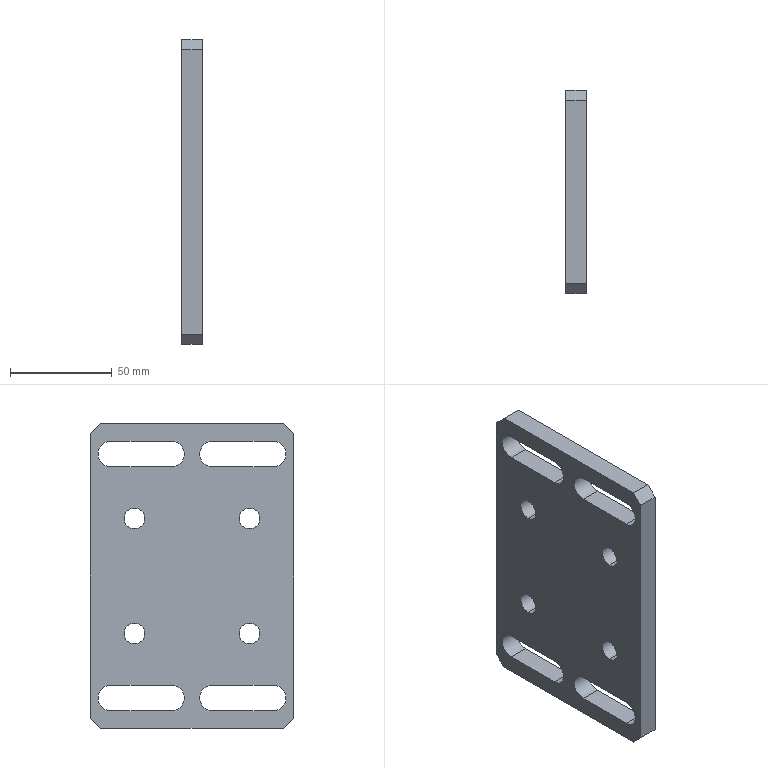Part | SolidWorks | features Chamfer 1, Extrusion 1, HoleWzd 1, ICE 1 | 1 solid | 34 faces | box 10 x 100 x 150 mm | volume 126323 mm3 | plane 18 | cylinder 16 | commonest cylinder face diameters 10.2 x8 12.5 x8
STEP:
#1=CARTESIAN_POINT('',(0.,28.284,33.384));
#2=VERTEX_POINT('',#1);
#3=CARTESIAN_POINT('',(0.,28.284,23.184));
#4=VERTEX_POINT('',#3);
#5=CARTESIAN_POINT('',(0.,28.284,28.284));
#6=DIRECTION('',(1.,0.,0.));
#7=DIRECTION('',(0.,0.,-1.));
#8=AXIS2_PLACEMENT_3D('',#5,#6,#7);
#9=CIRCLE('',#8,5.1);
#10=EDGE_CURVE('',#2,#4,#9,.T.);
#11=ORIENTED_EDGE('',*,*,#10,.F.);
#12=CARTESIAN_POINT('',(10.,28.284,33.384));
#13=VERTEX_POINT('',#12);
#14=CARTESIAN_POINT('',(10.,28.284,33.384));
#15=DIRECTION('',(1.,0.,0.));
#16=VECTOR('',#15,1000.);
#17=LINE('',#14,#16);
#18=EDGE_CURVE('',#2,#13,#17,.T.);
#19=ORIENTED_EDGE('',*,*,#18,.T.);
#20=CARTESIAN_POINT('',(10.,28.284,23.184));
#21=VERTEX_POINT('',#20);
#22=CARTESIAN_POINT('',(10.,28.284,28.284));
#23=DIRECTION('',(1.,0.,0.));
#24=DIRECTION('',(0.,0.,-1.));
#25=AXIS2_PLACEMENT_3D('',#22,#23,#24);
#26=CIRCLE('',#25,5.1);
#27=EDGE_CURVE('',#13,#21,#26,.T.);
#28=ORIENTED_EDGE('',*,*,#27,.T.);
#29=CARTESIAN_POINT('',(10.,28.284,23.184));
#30=DIRECTION('',(1.,0.,0.));
#31=VECTOR('',#30,1000.);
#32=LINE('',#29,#31);
#33=EDGE_CURVE('',#4,#21,#32,.T.);
#34=ORIENTED_EDGE('',*,*,#33,.F.);
#35=EDGE_LOOP('',(#11,#19,#28,#34));
#36=FACE_OUTER_BOUND('',#35,.T.);
#37=CARTESIAN_POINT('',(10.,28.284,28.284));
#38=DIRECTION('',(1.,0.,0.));
#39=DIRECTION('',(0.,0.,-1.));
#40=AXIS2_PLACEMENT_3D('',#37,#38,#39);
#41=CYLINDRICAL_SURFACE('',#40,5.1);
#42=ADVANCED_FACE('',(#36),#41,.F.);
#43=CARTESIAN_POINT('',(0.,28.284,-23.184));
#44=VERTEX_POINT('',#43);
#45=CARTESIAN_POINT('',(0.,28.284,-33.384));
#46=VERTEX_POINT('',#45);
#47=CARTESIAN_POINT('',(0.,28.284,-28.284));
#48=DIRECTION('',(1.,0.,0.));
#49=DIRECTION('',(0.,0.,-1.));
#50=AXIS2_PLACEMENT_3D('',#47,#48,#49);
#51=CIRCLE('',#50,5.1);
#52=EDGE_CURVE('',#44,#46,#51,.T.);
#53=ORIENTED_EDGE('',*,*,#52,.F.);
#54=CARTESIAN_POINT('',(10.,28.284,-23.184));
#55=VERTEX_POINT('',#54);
#56=CARTESIAN_POINT('',(10.,28.284,-23.184));
#57=DIRECTION('',(1.,0.,0.));
#58=VECTOR('',#57,1000.);
#59=LINE('',#56,#58);
#60=EDGE_CURVE('',#44,#55,#59,.T.);
#61=ORIENTED_EDGE('',*,*,#60,.T.);
#62=CARTESIAN_POINT('',(10.,28.284,-33.384));
#63=VERTEX_POINT('',#62);
#64=CARTESIAN_POINT('',(10.,28.284,-28.284));
#65=DIRECTION('',(1.,0.,0.));
#66=DIRECTION('',(0.,0.,-1.));
#67=AXIS2_PLACEMENT_3D('',#64,#65,#66);
#68=CIRCLE('',#67,5.1);
#69=EDGE_CURVE('',#55,#63,#68,.T.);
#70=ORIENTED_EDGE('',*,*,#69,.T.);
#71=CARTESIAN_POINT('',(10.,28.284,-33.384));
#72=DIRECTION('',(1.,0.,0.));
#73=VECTOR('',#72,1000.);
#74=LINE('',#71,#73);
#75=EDGE_CURVE('',#46,#63,#74,.T.);
#76=ORIENTED_EDGE('',*,*,#75,.F.);
#77=EDGE_LOOP('',(#53,#61,#70,#76));
#78=FACE_OUTER_BOUND('',#77,.T.);
#79=CARTESIAN_POINT('',(10.,28.284,-28.284));
#80=DIRECTION('',(1.,0.,0.));
#81=DIRECTION('',(0.,0.,-1.));
#82=AXIS2_PLACEMENT_3D('',#79,#80,#81);
#83=CYLINDRICAL_SURFACE('',#82,5.1);
#84=ADVANCED_FACE('',(#78),#83,.F.);
#85=CARTESIAN_POINT('',(0.,-28.284,-23.184));
#86=VERTEX_POINT('',#85);
#87=CARTESIAN_POINT('',(0.,-28.284,-33.384));
#88=VERTEX_POINT('',#87);
#89=CARTESIAN_POINT('',(0.,-28.284,-28.284));
#90=DIRECTION('',(1.,0.,0.));
#91=DIRECTION('',(0.,0.,-1.));
#92=AXIS2_PLACEMENT_3D('',#89,#90,#91);
#93=CIRCLE('',#92,5.1);
#94=EDGE_CURVE('',#86,#88,#93,.T.);
#95=ORIENTED_EDGE('',*,*,#94,.F.);
#96=CARTESIAN_POINT('',(10.,-28.284,-23.184));
#97=VERTEX_POINT('',#96);
#98=CARTESIAN_POINT('',(10.,-28.284,-23.184));
#99=DIRECTION('',(1.,0.,0.));
#100=VECTOR('',#99,1000.);
#101=LINE('',#98,#100);
#102=EDGE_CURVE('',#86,#97,#101,.T.);
#103=ORIENTED_EDGE('',*,*,#102,.T.);
#104=CARTESIAN_POINT('',(10.,-28.284,-33.384));
#105=VERTEX_POINT('',#104);
#106=CARTESIAN_POINT('',(10.,-28.284,-28.284));
#107=DIRECTION('',(1.,0.,0.));
#108=DIRECTION('',(0.,0.,-1.));
#109=AXIS2_PLACEMENT_3D('',#106,#107,#108);
#110=CIRCLE('',#109,5.1);
#111=EDGE_CURVE('',#97,#105,#110,.T.);
#112=ORIENTED_EDGE('',*,*,#111,.T.);
#113=CARTESIAN_POINT('',(10.,-28.284,-33.384));
#114=DIRECTION('',(1.,0.,0.));
#115=VECTOR('',#114,1000.);
#116=LINE('',#113,#115);
#117=EDGE_CURVE('',#88,#105,#116,.T.);
#118=ORIENTED_EDGE('',*,*,#117,.F.);
#119=EDGE_LOOP('',(#95,#103,#112,#118));
#120=FACE_OUTER_BOUND('',#119,.T.);
#121=CARTESIAN_POINT('',(10.,-28.284,-28.284));
#122=DIRECTION('',(1.,0.,0.));
#123=DIRECTION('',(0.,0.,-1.));
#124=AXIS2_PLACEMENT_3D('',#121,#122,#123);
#125=CYLINDRICAL_SURFACE('',#124,5.1);
#126=ADVANCED_FACE('',(#120),#125,.F.);
#127=CARTESIAN_POINT('',(0.,-28.284,33.384));
#128=VERTEX_POINT('',#127);
#129=CARTESIAN_POINT('',(0.,-28.284,23.184));
#130=VERTEX_POINT('',#129);
#131=CARTESIAN_POINT('',(0.,-28.284,28.284));
#132=DIRECTION('',(1.,0.,0.));
#133=DIRECTION('',(0.,0.,-1.));
#134=AXIS2_PLACEMENT_3D('',#131,#132,#133);
#135=CIRCLE('',#134,5.1);
#136=EDGE_CURVE('',#128,#130,#135,.T.);
#137=ORIENTED_EDGE('',*,*,#136,.F.);
#138=CARTESIAN_POINT('',(10.,-28.284,33.384));
#139=VERTEX_POINT('',#138);
#140=CARTESIAN_POINT('',(10.,-28.284,33.384));
#141=DIRECTION('',(1.,0.,0.));
#142=VECTOR('',#141,1000.);
#143=LINE('',#140,#142);
#144=EDGE_CURVE('',#128,#139,#143,.T.);
#145=ORIENTED_EDGE('',*,*,#144,.T.);
#146=CARTESIAN_POINT('',(10.,-28.284,23.184));
#147=VERTEX_POINT('',#146);
#148=CARTESIAN_POINT('',(10.,-28.284,28.284));
#149=DIRECTION('',(1.,0.,0.));
#150=DIRECTION('',(0.,0.,-1.));
#151=AXIS2_PLACEMENT_3D('',#148,#149,#150);
#152=CIRCLE('',#151,5.1);
#153=EDGE_CURVE('',#139,#147,#152,.T.);
#154=ORIENTED_EDGE('',*,*,#153,.T.);
#155=CARTESIAN_POINT('',(10.,-28.284,23.184));
#156=DIRECTION('',(1.,0.,0.));
#157=VECTOR('',#156,1000.);
#158=LINE('',#155,#157);
#159=EDGE_CURVE('',#130,#147,#158,.T.);
#160=ORIENTED_EDGE('',*,*,#159,.F.);
#161=EDGE_LOOP('',(#137,#145,#154,#160));
#162=FACE_OUTER_BOUND('',#161,.T.);
#163=CARTESIAN_POINT('',(10.,-28.284,28.284));
#164=DIRECTION('',(1.,0.,0.));
#165=DIRECTION('',(0.,0.,-1.));
#166=AXIS2_PLACEMENT_3D('',#163,#164,#165);
#167=CYLINDRICAL_SURFACE('',#166,5.1);
#168=ADVANCED_FACE('',(#162),#167,.F.);
#169=CARTESIAN_POINT('',(0.,-45.,-75.));
#170=VERTEX_POINT('',#169);
#171=CARTESIAN_POINT('',(0.,45.,-75.));
#172=VERTEX_POINT('',#171);
#173=CARTESIAN_POINT('',(0.,50.,-75.));
#174=DIRECTION('',(0.,1.,0.));
#175=VECTOR('',#174,1000.);
#176=LINE('',#173,#175);
#177=EDGE_CURVE('',#170,#172,#176,.T.);
#178=ORIENTED_EDGE('',*,*,#177,.T.);
#179=CARTESIAN_POINT('',(10.,45.,-75.));
#180=VERTEX_POINT('',#179);
#181=CARTESIAN_POINT('',(10.,45.,-75.));
#182=DIRECTION('',(1.,0.,0.));
#183=VECTOR('',#182,1000.);
#184=LINE('',#181,#183);
#185=EDGE_CURVE('',#172,#180,#184,.T.);
#186=ORIENTED_EDGE('',*,*,#185,.T.);
#187=CARTESIAN_POINT('',(10.,-45.,-75.));
#188=VERTEX_POINT('',#187);
#189=CARTESIAN_POINT('',(10.,50.,-75.));
#190=DIRECTION('',(0.,1.,0.));
#191=VECTOR('',#190,1000.);
#192=LINE('',#189,#191);
#193=EDGE_CURVE('',#188,#180,#192,.T.);
#194=ORIENTED_EDGE('',*,*,#193,.F.);
#195=CARTESIAN_POINT('',(10.,-45.,-75.));
#196=DIRECTION('',(-1.,0.,0.));
#197=VECTOR('',#196,1000.);
#198=LINE('',#195,#197);
#199=EDGE_CURVE('',#188,#170,#198,.T.);
#200=ORIENTED_EDGE('',*,*,#199,.T.);
#201=EDGE_LOOP('',(#178,#186,#194,#200));
#202=FACE_OUTER_BOUND('',#201,.T.);
#203=CARTESIAN_POINT('',(10.,50.,-75.));
#204=DIRECTION('',(0.,0.,1.));
#205=DIRECTION('',(0.,-1.,0.));
#206=AXIS2_PLACEMENT_3D('',#203,#204,#205);
#207=PLANE('',#206);
#208=ADVANCED_FACE('',(#202),#207,.F.);
#209=CARTESIAN_POINT('',(0.,50.,-70.));
#210=VERTEX_POINT('',#209);
#211=CARTESIAN_POINT('',(0.,50.,70.));
#212=VERTEX_POINT('',#211);
#213=CARTESIAN_POINT('',(0.,50.,75.));
#214=DIRECTION('',(0.,0.,1.));
#215=VECTOR('',#214,1000.);
#216=LINE('',#213,#215);
#217=EDGE_CURVE('',#210,#212,#216,.T.);
#218=ORIENTED_EDGE('',*,*,#217,.T.);
#219=CARTESIAN_POINT('',(10.,50.,70.));
#220=VERTEX_POINT('',#219);
#221=CARTESIAN_POINT('',(10.,50.,70.));
#222=DIRECTION('',(1.,0.,0.));
#223=VECTOR('',#222,1000.);
#224=LINE('',#221,#223);
#225=EDGE_CURVE('',#212,#220,#224,.T.);
#226=ORIENTED_EDGE('',*,*,#225,.T.);
#227=CARTESIAN_POINT('',(10.,50.,-70.));
#228=VERTEX_POINT('',#227);
#229=CARTESIAN_POINT('',(10.,50.,75.));
#230=DIRECTION('',(0.,0.,1.));
#231=VECTOR('',#230,1000.);
#232=LINE('',#229,#231);
#233=EDGE_CURVE('',#228,#220,#232,.T.);
#234=ORIENTED_EDGE('',*,*,#233,.F.);
#235=CARTESIAN_POINT('',(10.,50.,-70.));
#236=DIRECTION('',(-1.,0.,0.));
#237=VECTOR('',#236,1000.);
#238=LINE('',#235,#237);
#239=EDGE_CURVE('',#228,#210,#238,.T.);
#240=ORIENTED_EDGE('',*,*,#239,.T.);
#241=EDGE_LOOP('',(#218,#226,#234,#240));
#242=FACE_OUTER_BOUND('',#241,.T.);
#243=CARTESIAN_POINT('',(10.,50.,75.));
#244=DIRECTION('',(0.,-1.,0.));
#245=DIRECTION('',(0.,0.,-1.));
#246=AXIS2_PLACEMENT_3D('',#243,#244,#245);
#247=PLANE('',#246);
#248=ADVANCED_FACE('',(#242),#247,.F.);
#249=CARTESIAN_POINT('',(0.,45.,75.));
#250=VERTEX_POINT('',#249);
#251=CARTESIAN_POINT('',(0.,-45.,75.));
#252=VERTEX_POINT('',#251);
#253=CARTESIAN_POINT('',(0.,50.,75.));
#254=DIRECTION('',(0.,-1.,0.));
#255=VECTOR('',#254,1000.);
#256=LINE('',#253,#255);
#257=EDGE_CURVE('',#250,#252,#256,.T.);
#258=ORIENTED_EDGE('',*,*,#257,.T.);
#259=CARTESIAN_POINT('',(10.,-45.,75.));
#260=VERTEX_POINT('',#259);
#261=CARTESIAN_POINT('',(10.,-45.,75.));
#262=DIRECTION('',(1.,0.,0.));
#263=VECTOR('',#262,1000.);
#264=LINE('',#261,#263);
#265=EDGE_CURVE('',#252,#260,#264,.T.);
#266=ORIENTED_EDGE('',*,*,#265,.T.);
#267=CARTESIAN_POINT('',(10.,45.,75.));
#268=VERTEX_POINT('',#267);
#269=CARTESIAN_POINT('',(10.,50.,75.));
#270=DIRECTION('',(0.,-1.,0.));
#271=VECTOR('',#270,1000.);
#272=LINE('',#269,#271);
#273=EDGE_CURVE('',#268,#260,#272,.T.);
#274=ORIENTED_EDGE('',*,*,#273,.F.);
#275=CARTESIAN_POINT('',(10.,45.,75.));
#276=DIRECTION('',(-1.,0.,0.));
#277=VECTOR('',#276,1000.);
#278=LINE('',#275,#277);
#279=EDGE_CURVE('',#268,#250,#278,.T.);
#280=ORIENTED_EDGE('',*,*,#279,.T.);
#281=EDGE_LOOP('',(#258,#266,#274,#280));
#282=FACE_OUTER_BOUND('',#281,.T.);
#283=CARTESIAN_POINT('',(10.,50.,75.));
#284=DIRECTION('',(0.,0.,-1.));
#285=DIRECTION('',(0.,1.,0.));
#286=AXIS2_PLACEMENT_3D('',#283,#284,#285);
#287=PLANE('',#286);
#288=ADVANCED_FACE('',(#282),#287,.F.);
#289=CARTESIAN_POINT('',(10.,-50.,70.));
#290=VERTEX_POINT('',#289);
#291=CARTESIAN_POINT('',(10.,-50.,-70.));
#292=VERTEX_POINT('',#291);
#293=CARTESIAN_POINT('',(10.,-50.,75.));
#294=DIRECTION('',(0.,0.,-1.));
#295=VECTOR('',#294,1000.);
#296=LINE('',#293,#295);
#297=EDGE_CURVE('',#290,#292,#296,.T.);
#298=ORIENTED_EDGE('',*,*,#297,.F.);
#299=CARTESIAN_POINT('',(0.,-50.,70.));
#300=VERTEX_POINT('',#299);
#301=CARTESIAN_POINT('',(10.,-50.,70.));
#302=DIRECTION('',(-1.,0.,0.));
#303=VECTOR('',#302,1000.);
#304=LINE('',#301,#303);
#305=EDGE_CURVE('',#290,#300,#304,.T.);
#306=ORIENTED_EDGE('',*,*,#305,.T.);
#307=CARTESIAN_POINT('',(0.,-50.,-70.));
#308=VERTEX_POINT('',#307);
#309=CARTESIAN_POINT('',(0.,-50.,75.));
#310=DIRECTION('',(0.,0.,-1.));
#311=VECTOR('',#310,1000.);
#312=LINE('',#309,#311);
#313=EDGE_CURVE('',#300,#308,#312,.T.);
#314=ORIENTED_EDGE('',*,*,#313,.T.);
#315=CARTESIAN_POINT('',(10.,-50.,-70.));
#316=DIRECTION('',(1.,0.,0.));
#317=VECTOR('',#316,1000.);
#318=LINE('',#315,#317);
#319=EDGE_CURVE('',#308,#292,#318,.T.);
#320=ORIENTED_EDGE('',*,*,#319,.T.);
#321=EDGE_LOOP('',(#298,#306,#314,#320));
#322=FACE_OUTER_BOUND('',#321,.T.);
#323=CARTESIAN_POINT('',(10.,-50.,75.));
#324=DIRECTION('',(0.,1.,0.));
#325=DIRECTION('',(0.,0.,1.));
#326=AXIS2_PLACEMENT_3D('',#323,#324,#325);
#327=PLANE('',#326);
#328=ADVANCED_FACE('',(#322),#327,.F.);
#329=CARTESIAN_POINT('',(10.,40.,-66.25));
#330=VERTEX_POINT('',#329);
#331=CARTESIAN_POINT('',(10.,40.,-53.75));
#332=VERTEX_POINT('',#331);
#333=CARTESIAN_POINT('',(10.,40.,-60.));
#334=DIRECTION('',(1.,0.,0.));
#335=DIRECTION('',(0.,0.,1.));
#336=AXIS2_PLACEMENT_3D('',#333,#334,#335);
#337=CIRCLE('',#336,6.25);
#338=EDGE_CURVE('',#330,#332,#337,.T.);
#339=ORIENTED_EDGE('',*,*,#338,.F.);
#340=CARTESIAN_POINT('',(10.,10.,-66.25));
#341=VERTEX_POINT('',#340);
#342=CARTESIAN_POINT('',(10.,40.,-66.25));
#343=DIRECTION('',(0.,1.,0.));
#344=VECTOR('',#343,1000.);
#345=LINE('',#342,#344);
#346=EDGE_CURVE('',#341,#330,#345,.T.);
#347=ORIENTED_EDGE('',*,*,#346,.F.);
#348=CARTESIAN_POINT('',(10.,10.,-53.75));
#349=VERTEX_POINT('',#348);
#350=CARTESIAN_POINT('',(10.,10.,-60.));
#351=DIRECTION('',(1.,0.,0.));
#352=DIRECTION('',(0.,0.,1.));
#353=AXIS2_PLACEMENT_3D('',#350,#351,#352);
#354=CIRCLE('',#353,6.25);
#355=EDGE_CURVE('',#349,#341,#354,.T.);
#356=ORIENTED_EDGE('',*,*,#355,.F.);
#357=CARTESIAN_POINT('',(10.,40.,-53.75));
#358=DIRECTION('',(0.,-1.,0.));
#359=VECTOR('',#358,1000.);
#360=LINE('',#357,#359);
#361=EDGE_CURVE('',#332,#349,#360,.T.);
#362=ORIENTED_EDGE('',*,*,#361,.F.);
#363=EDGE_LOOP('',(#339,#347,#356,#362));
#364=FACE_BOUND('',#363,.T.);
#365=CARTESIAN_POINT('',(10.,-40.,66.25));
#366=VERTEX_POINT('',#365);
#367=CARTESIAN_POINT('',(10.,-40.,53.75));
#368=VERTEX_POINT('',#367);
#369=CARTESIAN_POINT('',(10.,-40.,60.));
#370=DIRECTION('',(1.,0.,0.));
#371=DIRECTION('',(0.,0.,1.));
#372=AXIS2_PLACEMENT_3D('',#369,#370,#371);
#373=CIRCLE('',#372,6.25);
#374=EDGE_CURVE('',#366,#368,#373,.T.);
#375=ORIENTED_EDGE('',*,*,#374,.F.);
#376=CARTESIAN_POINT('',(10.,-10.,66.25));
#377=VERTEX_POINT('',#376);
#378=CARTESIAN_POINT('',(10.,-40.,66.25));
#379=DIRECTION('',(0.,-1.,0.));
#380=VECTOR('',#379,1000.);
#381=LINE('',#378,#380);
#382=EDGE_CURVE('',#377,#366,#381,.T.);
#383=ORIENTED_EDGE('',*,*,#382,.F.);
#384=CARTESIAN_POINT('',(10.,-10.,53.75));
#385=VERTEX_POINT('',#384);
#386=CARTESIAN_POINT('',(10.,-10.,60.));
#387=DIRECTION('',(1.,0.,0.));
#388=DIRECTION('',(0.,0.,1.));
#389=AXIS2_PLACEMENT_3D('',#386,#387,#388);
#390=CIRCLE('',#389,6.25);
#391=EDGE_CURVE('',#385,#377,#390,.T.);
#392=ORIENTED_EDGE('',*,*,#391,.F.);
#393=CARTESIAN_POINT('',(10.,-40.,53.75));
#394=DIRECTION('',(0.,1.,0.));
#395=VECTOR('',#394,1000.);
#396=LINE('',#393,#395);
#397=EDGE_CURVE('',#368,#385,#396,.T.);
#398=ORIENTED_EDGE('',*,*,#397,.F.);
#399=EDGE_LOOP('',(#375,#383,#392,#398));
#400=FACE_BOUND('',#399,.T.);
#401=CARTESIAN_POINT('',(10.,-40.,-53.75));
#402=VERTEX_POINT('',#401);
#403=CARTESIAN_POINT('',(10.,-40.,-66.25));
#404=VERTEX_POINT('',#403);
#405=CARTESIAN_POINT('',(10.,-40.,-60.));
#406=DIRECTION('',(1.,0.,0.));
#407=DIRECTION('',(0.,0.,-1.));
#408=AXIS2_PLACEMENT_3D('',#405,#406,#407);
#409=CIRCLE('',#408,6.25);
#410=EDGE_CURVE('',#402,#404,#409,.T.);
#411=ORIENTED_EDGE('',*,*,#410,.F.);
#412=CARTESIAN_POINT('',(10.,-10.,-53.75));
#413=VERTEX_POINT('',#412);
#414=CARTESIAN_POINT('',(10.,-40.,-53.75));
#415=DIRECTION('',(0.,-1.,0.));
#416=VECTOR('',#415,1000.);
#417=LINE('',#414,#416);
#418=EDGE_CURVE('',#413,#402,#417,.T.);
#419=ORIENTED_EDGE('',*,*,#418,.F.);
#420=CARTESIAN_POINT('',(10.,-10.,-66.25));
#421=VERTEX_POINT('',#420);
#422=CARTESIAN_POINT('',(10.,-10.,-60.));
#423=DIRECTION('',(1.,0.,0.));
#424=DIRECTION('',(0.,0.,-1.));
#425=AXIS2_PLACEMENT_3D('',#422,#423,#424);
#426=CIRCLE('',#425,6.25);
#427=EDGE_CURVE('',#421,#413,#426,.T.);
#428=ORIENTED_EDGE('',*,*,#427,.F.);
#429=CARTESIAN_POINT('',(10.,-40.,-66.25));
#430=DIRECTION('',(0.,1.,0.));
#431=VECTOR('',#430,1000.);
#432=LINE('',#429,#431);
#433=EDGE_CURVE('',#404,#421,#432,.T.);
#434=ORIENTED_EDGE('',*,*,#433,.F.);
#435=EDGE_LOOP('',(#411,#419,#428,#434));
#436=FACE_BOUND('',#435,.T.);
#437=CARTESIAN_POINT('',(10.,40.,53.75));
#438=VERTEX_POINT('',#437);
#439=CARTESIAN_POINT('',(10.,40.,66.25));
#440=VERTEX_POINT('',#439);
#441=CARTESIAN_POINT('',(10.,40.,60.));
#442=DIRECTION('',(1.,0.,0.));
#443=DIRECTION('',(0.,0.,-1.));
#444=AXIS2_PLACEMENT_3D('',#441,#442,#443);
#445=CIRCLE('',#444,6.25);
#446=EDGE_CURVE('',#438,#440,#445,.T.);
#447=ORIENTED_EDGE('',*,*,#446,.F.);
#448=CARTESIAN_POINT('',(10.,10.,53.75));
#449=VERTEX_POINT('',#448);
#450=CARTESIAN_POINT('',(10.,40.,53.75));
#451=DIRECTION('',(0.,1.,0.));
#452=VECTOR('',#451,1000.);
#453=LINE('',#450,#452);
#454=EDGE_CURVE('',#449,#438,#453,.T.);
#455=ORIENTED_EDGE('',*,*,#454,.F.);
#456=CARTESIAN_POINT('',(10.,10.,66.25));
#457=VERTEX_POINT('',#456);
#458=CARTESIAN_POINT('',(10.,10.,60.));
#459=DIRECTION('',(1.,0.,0.));
#460=DIRECTION('',(0.,0.,-1.));
#461=AXIS2_PLACEMENT_3D('',#458,#459,#460);
#462=CIRCLE('',#461,6.25);
#463=EDGE_CURVE('',#457,#449,#462,.T.);
#464=ORIENTED_EDGE('',*,*,#463,.F.);
#465=CARTESIAN_POINT('',(10.,40.,66.25));
#466=DIRECTION('',(0.,-1.,0.));
#467=VECTOR('',#466,1000.);
#468=LINE('',#465,#467);
#469=EDGE_CURVE('',#440,#457,#468,.T.);
#470=ORIENTED_EDGE('',*,*,#469,.F.);
#471=EDGE_LOOP('',(#447,#455,#464,#470));
#472=FACE_BOUND('',#471,.T.);
#473=CARTESIAN_POINT('',(10.,28.284,28.284));
#474=DIRECTION('',(1.,0.,0.));
#475=DIRECTION('',(0.,0.,-1.));
#476=AXIS2_PLACEMENT_3D('',#473,#474,#475);
#477=CIRCLE('',#476,5.1);
#478=EDGE_CURVE('',#21,#13,#477,.T.);
#479=ORIENTED_EDGE('',*,*,#478,.F.);
#480=ORIENTED_EDGE('',*,*,#27,.F.);
#481=EDGE_LOOP('',(#479,#480));
#482=FACE_BOUND('',#481,.T.);
#483=CARTESIAN_POINT('',(10.,28.284,-28.284));
#484=DIRECTION('',(1.,0.,0.));
#485=DIRECTION('',(0.,0.,-1.));
#486=AXIS2_PLACEMENT_3D('',#483,#484,#485);
#487=CIRCLE('',#486,5.1);
#488=EDGE_CURVE('',#63,#55,#487,.T.);
#489=ORIENTED_EDGE('',*,*,#488,.F.);
#490=ORIENTED_EDGE('',*,*,#69,.F.);
#491=EDGE_LOOP('',(#489,#490));
#492=FACE_BOUND('',#491,.T.);
#493=CARTESIAN_POINT('',(10.,-28.284,-28.284));
#494=DIRECTION('',(1.,0.,0.));
#495=DIRECTION('',(0.,0.,-1.));
#496=AXIS2_PLACEMENT_3D('',#493,#494,#495);
#497=CIRCLE('',#496,5.1);
#498=EDGE_CURVE('',#105,#97,#497,.T.);
#499=ORIENTED_EDGE('',*,*,#498,.F.);
#500=ORIENTED_EDGE('',*,*,#111,.F.);
#501=EDGE_LOOP('',(#499,#500));
#502=FACE_BOUND('',#501,.T.);
#503=CARTESIAN_POINT('',(10.,-28.284,28.284));
#504=DIRECTION('',(1.,0.,0.));
#505=DIRECTION('',(0.,0.,-1.));
#506=AXIS2_PLACEMENT_3D('',#503,#504,#505);
#507=CIRCLE('',#506,5.1);
#508=EDGE_CURVE('',#147,#139,#507,.T.);
#509=ORIENTED_EDGE('',*,*,#508,.F.);
#510=ORIENTED_EDGE('',*,*,#153,.F.);
#511=EDGE_LOOP('',(#509,#510));
#512=FACE_BOUND('',#511,.T.);
#513=ORIENTED_EDGE('',*,*,#273,.T.);
#514=CARTESIAN_POINT('',(10.,-60.,60.));
#515=DIRECTION('',(0.,-0.7071,-0.7071));
#516=VECTOR('',#515,1000.);
#517=LINE('',#514,#516);
#518=EDGE_CURVE('',#260,#290,#517,.T.);
#519=ORIENTED_EDGE('',*,*,#518,.T.);
#520=ORIENTED_EDGE('',*,*,#297,.T.);
#521=CARTESIAN_POINT('',(10.,-60.,-60.));
#522=DIRECTION('',(0.,0.7071,-0.7071));
#523=VECTOR('',#522,1000.);
#524=LINE('',#521,#523);
#525=EDGE_CURVE('',#292,#188,#524,.T.);
#526=ORIENTED_EDGE('',*,*,#525,.T.);
#527=ORIENTED_EDGE('',*,*,#193,.T.);
#528=CARTESIAN_POINT('',(10.,60.,-60.));
#529=DIRECTION('',(0.,0.7071,0.7071));
#530=VECTOR('',#529,1000.);
#531=LINE('',#528,#530);
#532=EDGE_CURVE('',#180,#228,#531,.T.);
#533=ORIENTED_EDGE('',*,*,#532,.T.);
#534=ORIENTED_EDGE('',*,*,#233,.T.);
#535=CARTESIAN_POINT('',(10.,60.,60.));
#536=DIRECTION('',(0.,-0.7071,0.7071));
#537=VECTOR('',#536,1000.);
#538=LINE('',#535,#537);
#539=EDGE_CURVE('',#220,#268,#538,.T.);
#540=ORIENTED_EDGE('',*,*,#539,.T.);
#541=EDGE_LOOP('',(#513,#519,#520,#526,#527,#533,#534,#540));
#542=FACE_OUTER_BOUND('',#541,.T.);
#543=CARTESIAN_POINT('',(10.,0.,0.));
#544=DIRECTION('',(1.,0.,0.));
#545=DIRECTION('',(0.,0.,-1.));
#546=AXIS2_PLACEMENT_3D('',#543,#544,#545);
#547=PLANE('',#546);
#548=ADVANCED_FACE('',(#364,#400,#436,#472,#482,#492,#502,#512,#542),#547,.T.);
#549=CARTESIAN_POINT('',(0.,10.,-66.25));
#550=VERTEX_POINT('',#549);
#551=CARTESIAN_POINT('',(0.,40.,-66.25));
#552=VERTEX_POINT('',#551);
#553=CARTESIAN_POINT('',(0.,40.,-66.25));
#554=DIRECTION('',(0.,1.,0.));
#555=VECTOR('',#554,1000.);
#556=LINE('',#553,#555);
#557=EDGE_CURVE('',#550,#552,#556,.T.);
#558=ORIENTED_EDGE('',*,*,#557,.T.);
#559=CARTESIAN_POINT('',(0.,40.,-53.75));
#560=VERTEX_POINT('',#559);
#561=CARTESIAN_POINT('',(0.,40.,-60.));
#562=DIRECTION('',(1.,0.,0.));
#563=DIRECTION('',(0.,0.,1.));
#564=AXIS2_PLACEMENT_3D('',#561,#562,#563);
#565=CIRCLE('',#564,6.25);
#566=EDGE_CURVE('',#552,#560,#565,.T.);
#567=ORIENTED_EDGE('',*,*,#566,.T.);
#568=CARTESIAN_POINT('',(0.,10.,-53.75));
#569=VERTEX_POINT('',#568);
#570=CARTESIAN_POINT('',(0.,40.,-53.75));
#571=DIRECTION('',(0.,-1.,0.));
#572=VECTOR('',#571,1000.);
#573=LINE('',#570,#572);
#574=EDGE_CURVE('',#560,#569,#573,.T.);
#575=ORIENTED_EDGE('',*,*,#574,.T.);
#576=CARTESIAN_POINT('',(0.,10.,-60.));
#577=DIRECTION('',(1.,0.,0.));
#578=DIRECTION('',(0.,0.,1.));
#579=AXIS2_PLACEMENT_3D('',#576,#577,#578);
#580=CIRCLE('',#579,6.25);
#581=EDGE_CURVE('',#569,#550,#580,.T.);
#582=ORIENTED_EDGE('',*,*,#581,.T.);
#583=EDGE_LOOP('',(#558,#567,#575,#582));
#584=FACE_BOUND('',#583,.T.);
#585=CARTESIAN_POINT('',(0.,-10.,66.25));
#586=VERTEX_POINT('',#585);
#587=CARTESIAN_POINT('',(0.,-40.,66.25));
#588=VERTEX_POINT('',#587);
#589=CARTESIAN_POINT('',(0.,-40.,66.25));
#590=DIRECTION('',(0.,-1.,0.));
#591=VECTOR('',#590,1000.);
#592=LINE('',#589,#591);
#593=EDGE_CURVE('',#586,#588,#592,.T.);
#594=ORIENTED_EDGE('',*,*,#593,.T.);
#595=CARTESIAN_POINT('',(0.,-40.,53.75));
#596=VERTEX_POINT('',#595);
#597=CARTESIAN_POINT('',(0.,-40.,60.));
#598=DIRECTION('',(1.,0.,0.));
#599=DIRECTION('',(0.,0.,1.));
#600=AXIS2_PLACEMENT_3D('',#597,#598,#599);
#601=CIRCLE('',#600,6.25);
#602=EDGE_CURVE('',#588,#596,#601,.T.);
#603=ORIENTED_EDGE('',*,*,#602,.T.);
#604=CARTESIAN_POINT('',(0.,-10.,53.75));
#605=VERTEX_POINT('',#604);
#606=CARTESIAN_POINT('',(0.,-40.,53.75));
#607=DIRECTION('',(0.,1.,0.));
#608=VECTOR('',#607,1000.);
#609=LINE('',#606,#608);
#610=EDGE_CURVE('',#596,#605,#609,.T.);
#611=ORIENTED_EDGE('',*,*,#610,.T.);
#612=CARTESIAN_POINT('',(0.,-10.,60.));
#613=DIRECTION('',(1.,0.,0.));
#614=DIRECTION('',(0.,0.,1.));
#615=AXIS2_PLACEMENT_3D('',#612,#613,#614);
#616=CIRCLE('',#615,6.25);
#617=EDGE_CURVE('',#605,#586,#616,.T.);
#618=ORIENTED_EDGE('',*,*,#617,.T.);
#619=EDGE_LOOP('',(#594,#603,#611,#618));
#620=FACE_BOUND('',#619,.T.);
#621=CARTESIAN_POINT('',(0.,-10.,-53.75));
#622=VERTEX_POINT('',#621);
#623=CARTESIAN_POINT('',(0.,-40.,-53.75));
#624=VERTEX_POINT('',#623);
#625=CARTESIAN_POINT('',(0.,-40.,-53.75));
#626=DIRECTION('',(0.,-1.,0.));
#627=VECTOR('',#626,1000.);
#628=LINE('',#625,#627);
#629=EDGE_CURVE('',#622,#624,#628,.T.);
#630=ORIENTED_EDGE('',*,*,#629,.T.);
#631=CARTESIAN_POINT('',(0.,-40.,-66.25));
#632=VERTEX_POINT('',#631);
#633=CARTESIAN_POINT('',(0.,-40.,-60.));
#634=DIRECTION('',(1.,0.,0.));
#635=DIRECTION('',(0.,0.,-1.));
#636=AXIS2_PLACEMENT_3D('',#633,#634,#635);
#637=CIRCLE('',#636,6.25);
#638=EDGE_CURVE('',#624,#632,#637,.T.);
#639=ORIENTED_EDGE('',*,*,#638,.T.);
#640=CARTESIAN_POINT('',(0.,-10.,-66.25));
#641=VERTEX_POINT('',#640);
#642=CARTESIAN_POINT('',(0.,-40.,-66.25));
#643=DIRECTION('',(0.,1.,0.));
#644=VECTOR('',#643,1000.);
#645=LINE('',#642,#644);
#646=EDGE_CURVE('',#632,#641,#645,.T.);
#647=ORIENTED_EDGE('',*,*,#646,.T.);
#648=CARTESIAN_POINT('',(0.,-10.,-60.));
#649=DIRECTION('',(1.,0.,0.));
#650=DIRECTION('',(0.,0.,-1.));
#651=AXIS2_PLACEMENT_3D('',#648,#649,#650);
#652=CIRCLE('',#651,6.25);
#653=EDGE_CURVE('',#641,#622,#652,.T.);
#654=ORIENTED_EDGE('',*,*,#653,.T.);
#655=EDGE_LOOP('',(#630,#639,#647,#654));
#656=FACE_BOUND('',#655,.T.);
#657=CARTESIAN_POINT('',(0.,10.,53.75));
#658=VERTEX_POINT('',#657);
#659=CARTESIAN_POINT('',(0.,40.,53.75));
#660=VERTEX_POINT('',#659);
#661=CARTESIAN_POINT('',(0.,40.,53.75));
#662=DIRECTION('',(0.,1.,0.));
#663=VECTOR('',#662,1000.);
#664=LINE('',#661,#663);
#665=EDGE_CURVE('',#658,#660,#664,.T.);
#666=ORIENTED_EDGE('',*,*,#665,.T.);
#667=CARTESIAN_POINT('',(0.,40.,66.25));
#668=VERTEX_POINT('',#667);
#669=CARTESIAN_POINT('',(0.,40.,60.));
#670=DIRECTION('',(1.,0.,0.));
#671=DIRECTION('',(0.,0.,-1.));
#672=AXIS2_PLACEMENT_3D('',#669,#670,#671);
#673=CIRCLE('',#672,6.25);
#674=EDGE_CURVE('',#660,#668,#673,.T.);
#675=ORIENTED_EDGE('',*,*,#674,.T.);
#676=CARTESIAN_POINT('',(0.,10.,66.25));
#677=VERTEX_POINT('',#676);
#678=CARTESIAN_POINT('',(0.,40.,66.25));
#679=DIRECTION('',(0.,-1.,0.));
#680=VECTOR('',#679,1000.);
#681=LINE('',#678,#680);
#682=EDGE_CURVE('',#668,#677,#681,.T.);
#683=ORIENTED_EDGE('',*,*,#682,.T.);
#684=CARTESIAN_POINT('',(0.,10.,60.));
#685=DIRECTION('',(1.,0.,0.));
#686=DIRECTION('',(0.,0.,-1.));
#687=AXIS2_PLACEMENT_3D('',#684,#685,#686);
#688=CIRCLE('',#687,6.25);
#689=EDGE_CURVE('',#677,#658,#688,.T.);
#690=ORIENTED_EDGE('',*,*,#689,.T.);
#691=EDGE_LOOP('',(#666,#675,#683,#690));
#692=FACE_BOUND('',#691,.T.);
#693=CARTESIAN_POINT('',(0.,28.284,28.284));
#694=DIRECTION('',(1.,0.,0.));
#695=DIRECTION('',(0.,0.,-1.));
#696=AXIS2_PLACEMENT_3D('',#693,#694,#695);
#697=CIRCLE('',#696,5.1);
#698=EDGE_CURVE('',#4,#2,#697,.T.);
#699=ORIENTED_EDGE('',*,*,#698,.T.);
#700=ORIENTED_EDGE('',*,*,#10,.T.);
#701=EDGE_LOOP('',(#699,#700));
#702=FACE_BOUND('',#701,.T.);
#703=CARTESIAN_POINT('',(0.,28.284,-28.284));
#704=DIRECTION('',(1.,0.,0.));
#705=DIRECTION('',(0.,0.,-1.));
#706=AXIS2_PLACEMENT_3D('',#703,#704,#705);
#707=CIRCLE('',#706,5.1);
#708=EDGE_CURVE('',#46,#44,#707,.T.);
#709=ORIENTED_EDGE('',*,*,#708,.T.);
#710=ORIENTED_EDGE('',*,*,#52,.T.);
#711=EDGE_LOOP('',(#709,#710));
#712=FACE_BOUND('',#711,.T.);
#713=CARTESIAN_POINT('',(0.,-28.284,-28.284));
#714=DIRECTION('',(1.,0.,0.));
#715=DIRECTION('',(0.,0.,-1.));
#716=AXIS2_PLACEMENT_3D('',#713,#714,#715);
#717=CIRCLE('',#716,5.1);
#718=EDGE_CURVE('',#88,#86,#717,.T.);
#719=ORIENTED_EDGE('',*,*,#718,.T.);
#720=ORIENTED_EDGE('',*,*,#94,.T.);
#721=EDGE_LOOP('',(#719,#720));
#722=FACE_BOUND('',#721,.T.);
#723=CARTESIAN_POINT('',(0.,-28.284,28.284));
#724=DIRECTION('',(1.,0.,0.));
#725=DIRECTION('',(0.,0.,-1.));
#726=AXIS2_PLACEMENT_3D('',#723,#724,#725);
#727=CIRCLE('',#726,5.1);
#728=EDGE_CURVE('',#130,#128,#727,.T.);
#729=ORIENTED_EDGE('',*,*,#728,.T.);
#730=ORIENTED_EDGE('',*,*,#136,.T.);
#731=EDGE_LOOP('',(#729,#730));
#732=FACE_BOUND('',#731,.T.);
#733=ORIENTED_EDGE('',*,*,#313,.F.);
#734=CARTESIAN_POINT('',(0.,-50.,70.));
#735=DIRECTION('',(0.,0.7071,0.7071));
#736=VECTOR('',#735,1000.);
#737=LINE('',#734,#736);
#738=EDGE_CURVE('',#300,#252,#737,.T.);
#739=ORIENTED_EDGE('',*,*,#738,.T.);
#740=ORIENTED_EDGE('',*,*,#257,.F.);
#741=CARTESIAN_POINT('',(0.,45.,75.));
#742=DIRECTION('',(0.,0.7071,-0.7071));
#743=VECTOR('',#742,1000.);
#744=LINE('',#741,#743);
#745=EDGE_CURVE('',#250,#212,#744,.T.);
#746=ORIENTED_EDGE('',*,*,#745,.T.);
#747=ORIENTED_EDGE('',*,*,#217,.F.);
#748=CARTESIAN_POINT('',(0.,50.,-70.));
#749=DIRECTION('',(0.,-0.7071,-0.7071));
#750=VECTOR('',#749,1000.);
#751=LINE('',#748,#750);
#752=EDGE_CURVE('',#210,#172,#751,.T.);
#753=ORIENTED_EDGE('',*,*,#752,.T.);
#754=ORIENTED_EDGE('',*,*,#177,.F.);
#755=CARTESIAN_POINT('',(0.,-45.,-75.));
#756=DIRECTION('',(0.,-0.7071,0.7071));
#757=VECTOR('',#756,1000.);
#758=LINE('',#755,#757);
#759=EDGE_CURVE('',#170,#308,#758,.T.);
#760=ORIENTED_EDGE('',*,*,#759,.T.);
#761=EDGE_LOOP('',(#733,#739,#740,#746,#747,#753,#754,#760));
#762=FACE_OUTER_BOUND('',#761,.T.);
#763=CARTESIAN_POINT('',(0.,0.,0.));
#764=DIRECTION('',(1.,0.,0.));
#765=DIRECTION('',(0.,0.,-1.));
#766=AXIS2_PLACEMENT_3D('',#763,#764,#765);
#767=PLANE('',#766);
#768=ADVANCED_FACE('',(#584,#620,#656,#692,#702,#712,#722,#732,#762),#767,.F.);
#769=ORIENTED_EDGE('',*,*,#144,.F.);
#770=ORIENTED_EDGE('',*,*,#728,.F.);
#771=ORIENTED_EDGE('',*,*,#159,.T.);
#772=ORIENTED_EDGE('',*,*,#508,.T.);
#773=EDGE_LOOP('',(#769,#770,#771,#772));
#774=FACE_OUTER_BOUND('',#773,.T.);
#775=CARTESIAN_POINT('',(10.,-28.284,28.284));
#776=DIRECTION('',(1.,0.,0.));
#777=DIRECTION('',(0.,0.,-1.));
#778=AXIS2_PLACEMENT_3D('',#775,#776,#777);
#779=CYLINDRICAL_SURFACE('',#778,5.1);
#780=ADVANCED_FACE('',(#774),#779,.F.);
#781=ORIENTED_EDGE('',*,*,#102,.F.);
#782=ORIENTED_EDGE('',*,*,#718,.F.);
#783=ORIENTED_EDGE('',*,*,#117,.T.);
#784=ORIENTED_EDGE('',*,*,#498,.T.);
#785=EDGE_LOOP('',(#781,#782,#783,#784));
#786=FACE_OUTER_BOUND('',#785,.T.);
#787=CARTESIAN_POINT('',(10.,-28.284,-28.284));
#788=DIRECTION('',(1.,0.,0.));
#789=DIRECTION('',(0.,0.,-1.));
#790=AXIS2_PLACEMENT_3D('',#787,#788,#789);
#791=CYLINDRICAL_SURFACE('',#790,5.1);
#792=ADVANCED_FACE('',(#786),#791,.F.);
#793=ORIENTED_EDGE('',*,*,#60,.F.);
#794=ORIENTED_EDGE('',*,*,#708,.F.);
#795=ORIENTED_EDGE('',*,*,#75,.T.);
#796=ORIENTED_EDGE('',*,*,#488,.T.);
#797=EDGE_LOOP('',(#793,#794,#795,#796));
#798=FACE_OUTER_BOUND('',#797,.T.);
#799=CARTESIAN_POINT('',(10.,28.284,-28.284));
#800=DIRECTION('',(1.,0.,0.));
#801=DIRECTION('',(0.,0.,-1.));
#802=AXIS2_PLACEMENT_3D('',#799,#800,#801);
#803=CYLINDRICAL_SURFACE('',#802,5.1);
#804=ADVANCED_FACE('',(#798),#803,.F.);
#805=ORIENTED_EDGE('',*,*,#18,.F.);
#806=ORIENTED_EDGE('',*,*,#698,.F.);
#807=ORIENTED_EDGE('',*,*,#33,.T.);
#808=ORIENTED_EDGE('',*,*,#478,.T.);
#809=EDGE_LOOP('',(#805,#806,#807,#808));
#810=FACE_OUTER_BOUND('',#809,.T.);
#811=CARTESIAN_POINT('',(10.,28.284,28.284));
#812=DIRECTION('',(1.,0.,0.));
#813=DIRECTION('',(0.,0.,-1.));
#814=AXIS2_PLACEMENT_3D('',#811,#812,#813);
#815=CYLINDRICAL_SURFACE('',#814,5.1);
#816=ADVANCED_FACE('',(#810),#815,.F.);
#817=ORIENTED_EDGE('',*,*,#446,.T.);
#818=CARTESIAN_POINT('',(0.,40.,66.25));
#819=DIRECTION('',(1.,0.,0.));
#820=VECTOR('',#819,1000.);
#821=LINE('',#818,#820);
#822=EDGE_CURVE('',#668,#440,#821,.T.);
#823=ORIENTED_EDGE('',*,*,#822,.F.);
#824=ORIENTED_EDGE('',*,*,#674,.F.);
#825=CARTESIAN_POINT('',(0.,40.,53.75));
#826=DIRECTION('',(1.,0.,0.));
#827=VECTOR('',#826,1000.);
#828=LINE('',#825,#827);
#829=EDGE_CURVE('',#660,#438,#828,.T.);
#830=ORIENTED_EDGE('',*,*,#829,.T.);
#831=EDGE_LOOP('',(#817,#823,#824,#830));
#832=FACE_OUTER_BOUND('',#831,.T.);
#833=CARTESIAN_POINT('',(0.,40.,60.));
#834=DIRECTION('',(1.,0.,0.));
#835=DIRECTION('',(0.,0.,-1.));
#836=AXIS2_PLACEMENT_3D('',#833,#834,#835);
#837=CYLINDRICAL_SURFACE('',#836,6.25);
#838=ADVANCED_FACE('',(#832),#837,.F.);
#839=ORIENTED_EDGE('',*,*,#454,.T.);
#840=ORIENTED_EDGE('',*,*,#829,.F.);
#841=ORIENTED_EDGE('',*,*,#665,.F.);
#842=CARTESIAN_POINT('',(0.,10.,53.75));
#843=DIRECTION('',(1.,0.,0.));
#844=VECTOR('',#843,1000.);
#845=LINE('',#842,#844);
#846=EDGE_CURVE('',#658,#449,#845,.T.);
#847=ORIENTED_EDGE('',*,*,#846,.T.);
#848=EDGE_LOOP('',(#839,#840,#841,#847));
#849=FACE_OUTER_BOUND('',#848,.T.);
#850=CARTESIAN_POINT('',(0.,40.,53.75));
#851=DIRECTION('',(0.,0.,-1.));
#852=DIRECTION('',(-1.,0.,0.));
#853=AXIS2_PLACEMENT_3D('',#850,#851,#852);
#854=PLANE('',#853);
#855=ADVANCED_FACE('',(#849),#854,.F.);
#856=ORIENTED_EDGE('',*,*,#463,.T.);
#857=ORIENTED_EDGE('',*,*,#846,.F.);
#858=ORIENTED_EDGE('',*,*,#689,.F.);
#859=CARTESIAN_POINT('',(0.,10.,66.25));
#860=DIRECTION('',(1.,0.,0.));
#861=VECTOR('',#860,1000.);
#862=LINE('',#859,#861);
#863=EDGE_CURVE('',#677,#457,#862,.T.);
#864=ORIENTED_EDGE('',*,*,#863,.T.);
#865=EDGE_LOOP('',(#856,#857,#858,#864));
#866=FACE_OUTER_BOUND('',#865,.T.);
#867=CARTESIAN_POINT('',(0.,10.,60.));
#868=DIRECTION('',(1.,0.,0.));
#869=DIRECTION('',(0.,0.,-1.));
#870=AXIS2_PLACEMENT_3D('',#867,#868,#869);
#871=CYLINDRICAL_SURFACE('',#870,6.25);
#872=ADVANCED_FACE('',(#866),#871,.F.);
#873=ORIENTED_EDGE('',*,*,#469,.T.);
#874=ORIENTED_EDGE('',*,*,#863,.F.);
#875=ORIENTED_EDGE('',*,*,#682,.F.);
#876=ORIENTED_EDGE('',*,*,#822,.T.);
#877=EDGE_LOOP('',(#873,#874,#875,#876));
#878=FACE_OUTER_BOUND('',#877,.T.);
#879=CARTESIAN_POINT('',(0.,40.,66.25));
#880=DIRECTION('',(0.,0.,1.));
#881=DIRECTION('',(1.,0.,0.));
#882=AXIS2_PLACEMENT_3D('',#879,#880,#881);
#883=PLANE('',#882);
#884=ADVANCED_FACE('',(#878),#883,.F.);
#885=ORIENTED_EDGE('',*,*,#410,.T.);
#886=CARTESIAN_POINT('',(0.,-40.,-66.25));
#887=DIRECTION('',(1.,0.,0.));
#888=VECTOR('',#887,1000.);
#889=LINE('',#886,#888);
#890=EDGE_CURVE('',#632,#404,#889,.T.);
#891=ORIENTED_EDGE('',*,*,#890,.F.);
#892=ORIENTED_EDGE('',*,*,#638,.F.);
#893=CARTESIAN_POINT('',(0.,-40.,-53.75));
#894=DIRECTION('',(1.,0.,0.));
#895=VECTOR('',#894,1000.);
#896=LINE('',#893,#895);
#897=EDGE_CURVE('',#624,#402,#896,.T.);
#898=ORIENTED_EDGE('',*,*,#897,.T.);
#899=EDGE_LOOP('',(#885,#891,#892,#898));
#900=FACE_OUTER_BOUND('',#899,.T.);
#901=CARTESIAN_POINT('',(0.,-40.,-60.));
#902=DIRECTION('',(1.,0.,0.));
#903=DIRECTION('',(0.,0.,-1.));
#904=AXIS2_PLACEMENT_3D('',#901,#902,#903);
#905=CYLINDRICAL_SURFACE('',#904,6.25);
#906=ADVANCED_FACE('',(#900),#905,.F.);
#907=ORIENTED_EDGE('',*,*,#418,.T.);
#908=ORIENTED_EDGE('',*,*,#897,.F.);
#909=ORIENTED_EDGE('',*,*,#629,.F.);
#910=CARTESIAN_POINT('',(0.,-10.,-53.75));
#911=DIRECTION('',(1.,0.,0.));
#912=VECTOR('',#911,1000.);
#913=LINE('',#910,#912);
#914=EDGE_CURVE('',#622,#413,#913,.T.);
#915=ORIENTED_EDGE('',*,*,#914,.T.);
#916=EDGE_LOOP('',(#907,#908,#909,#915));
#917=FACE_OUTER_BOUND('',#916,.T.);
#918=CARTESIAN_POINT('',(0.,-40.,-53.75));
#919=DIRECTION('',(0.,0.,1.));
#920=DIRECTION('',(1.,0.,0.));
#921=AXIS2_PLACEMENT_3D('',#918,#919,#920);
#922=PLANE('',#921);
#923=ADVANCED_FACE('',(#917),#922,.F.);
#924=ORIENTED_EDGE('',*,*,#427,.T.);
#925=ORIENTED_EDGE('',*,*,#914,.F.);
#926=ORIENTED_EDGE('',*,*,#653,.F.);
#927=CARTESIAN_POINT('',(0.,-10.,-66.25));
#928=DIRECTION('',(1.,0.,0.));
#929=VECTOR('',#928,1000.);
#930=LINE('',#927,#929);
#931=EDGE_CURVE('',#641,#421,#930,.T.);
#932=ORIENTED_EDGE('',*,*,#931,.T.);
#933=EDGE_LOOP('',(#924,#925,#926,#932));
#934=FACE_OUTER_BOUND('',#933,.T.);
#935=CARTESIAN_POINT('',(0.,-10.,-60.));
#936=DIRECTION('',(1.,0.,0.));
#937=DIRECTION('',(0.,0.,-1.));
#938=AXIS2_PLACEMENT_3D('',#935,#936,#937);
#939=CYLINDRICAL_SURFACE('',#938,6.25);
#940=ADVANCED_FACE('',(#934),#939,.F.);
#941=ORIENTED_EDGE('',*,*,#433,.T.);
#942=ORIENTED_EDGE('',*,*,#931,.F.);
#943=ORIENTED_EDGE('',*,*,#646,.F.);
#944=ORIENTED_EDGE('',*,*,#890,.T.);
#945=EDGE_LOOP('',(#941,#942,#943,#944));
#946=FACE_OUTER_BOUND('',#945,.T.);
#947=CARTESIAN_POINT('',(0.,-40.,-66.25));
#948=DIRECTION('',(0.,0.,-1.));
#949=DIRECTION('',(-1.,0.,0.));
#950=AXIS2_PLACEMENT_3D('',#947,#948,#949);
#951=PLANE('',#950);
#952=ADVANCED_FACE('',(#946),#951,.F.);
#953=ORIENTED_EDGE('',*,*,#374,.T.);
#954=CARTESIAN_POINT('',(0.,-40.,53.75));
#955=DIRECTION('',(1.,0.,0.));
#956=VECTOR('',#955,1000.);
#957=LINE('',#954,#956);
#958=EDGE_CURVE('',#596,#368,#957,.T.);
#959=ORIENTED_EDGE('',*,*,#958,.F.);
#960=ORIENTED_EDGE('',*,*,#602,.F.);
#961=CARTESIAN_POINT('',(0.,-40.,66.25));
#962=DIRECTION('',(1.,0.,0.));
#963=VECTOR('',#962,1000.);
#964=LINE('',#961,#963);
#965=EDGE_CURVE('',#588,#366,#964,.T.);
#966=ORIENTED_EDGE('',*,*,#965,.T.);
#967=EDGE_LOOP('',(#953,#959,#960,#966));
#968=FACE_OUTER_BOUND('',#967,.T.);
#969=CARTESIAN_POINT('',(0.,-40.,60.));
#970=DIRECTION('',(1.,0.,0.));
#971=DIRECTION('',(0.,0.,-1.));
#972=AXIS2_PLACEMENT_3D('',#969,#970,#971);
#973=CYLINDRICAL_SURFACE('',#972,6.25);
#974=ADVANCED_FACE('',(#968),#973,.F.);
#975=ORIENTED_EDGE('',*,*,#382,.T.);
#976=ORIENTED_EDGE('',*,*,#965,.F.);
#977=ORIENTED_EDGE('',*,*,#593,.F.);
#978=CARTESIAN_POINT('',(0.,-10.,66.25));
#979=DIRECTION('',(1.,0.,0.));
#980=VECTOR('',#979,1000.);
#981=LINE('',#978,#980);
#982=EDGE_CURVE('',#586,#377,#981,.T.);
#983=ORIENTED_EDGE('',*,*,#982,.T.);
#984=EDGE_LOOP('',(#975,#976,#977,#983));
#985=FACE_OUTER_BOUND('',#984,.T.);
#986=CARTESIAN_POINT('',(0.,-40.,66.25));
#987=DIRECTION('',(0.,0.,1.));
#988=DIRECTION('',(1.,0.,0.));
#989=AXIS2_PLACEMENT_3D('',#986,#987,#988);
#990=PLANE('',#989);
#991=ADVANCED_FACE('',(#985),#990,.F.);
#992=ORIENTED_EDGE('',*,*,#391,.T.);
#993=ORIENTED_EDGE('',*,*,#982,.F.);
#994=ORIENTED_EDGE('',*,*,#617,.F.);
#995=CARTESIAN_POINT('',(0.,-10.,53.75));
#996=DIRECTION('',(1.,0.,0.));
#997=VECTOR('',#996,1000.);
#998=LINE('',#995,#997);
#999=EDGE_CURVE('',#605,#385,#998,.T.);
#1000=ORIENTED_EDGE('',*,*,#999,.T.);
#1001=EDGE_LOOP('',(#992,#993,#994,#1000));
#1002=FACE_OUTER_BOUND('',#1001,.T.);
#1003=CARTESIAN_POINT('',(0.,-10.,60.));
#1004=DIRECTION('',(1.,0.,0.));
#1005=DIRECTION('',(0.,0.,-1.));
#1006=AXIS2_PLACEMENT_3D('',#1003,#1004,#1005);
#1007=CYLINDRICAL_SURFACE('',#1006,6.25);
#1008=ADVANCED_FACE('',(#1002),#1007,.F.);
#1009=ORIENTED_EDGE('',*,*,#397,.T.);
#1010=ORIENTED_EDGE('',*,*,#999,.F.);
#1011=ORIENTED_EDGE('',*,*,#610,.F.);
#1012=ORIENTED_EDGE('',*,*,#958,.T.);
#1013=EDGE_LOOP('',(#1009,#1010,#1011,#1012));
#1014=FACE_OUTER_BOUND('',#1013,.T.);
#1015=CARTESIAN_POINT('',(0.,-40.,53.75));
#1016=DIRECTION('',(0.,0.,-1.));
#1017=DIRECTION('',(-1.,0.,0.));
#1018=AXIS2_PLACEMENT_3D('',#1015,#1016,#1017);
#1019=PLANE('',#1018);
#1020=ADVANCED_FACE('',(#1014),#1019,.F.);
#1021=ORIENTED_EDGE('',*,*,#338,.T.);
#1022=CARTESIAN_POINT('',(0.,40.,-53.75));
#1023=DIRECTION('',(1.,0.,0.));
#1024=VECTOR('',#1023,1000.);
#1025=LINE('',#1022,#1024);
#1026=EDGE_CURVE('',#560,#332,#1025,.T.);
#1027=ORIENTED_EDGE('',*,*,#1026,.F.);
#1028=ORIENTED_EDGE('',*,*,#566,.F.);
#1029=CARTESIAN_POINT('',(0.,40.,-66.25));
#1030=DIRECTION('',(1.,0.,0.));
#1031=VECTOR('',#1030,1000.);
#1032=LINE('',#1029,#1031);
#1033=EDGE_CURVE('',#552,#330,#1032,.T.);
#1034=ORIENTED_EDGE('',*,*,#1033,.T.);
#1035=EDGE_LOOP('',(#1021,#1027,#1028,#1034));
#1036=FACE_OUTER_BOUND('',#1035,.T.);
#1037=CARTESIAN_POINT('',(0.,40.,-60.));
#1038=DIRECTION('',(1.,0.,0.));
#1039=DIRECTION('',(0.,0.,-1.));
#1040=AXIS2_PLACEMENT_3D('',#1037,#1038,#1039);
#1041=CYLINDRICAL_SURFACE('',#1040,6.25);
#1042=ADVANCED_FACE('',(#1036),#1041,.F.);
#1043=ORIENTED_EDGE('',*,*,#346,.T.);
#1044=ORIENTED_EDGE('',*,*,#1033,.F.);
#1045=ORIENTED_EDGE('',*,*,#557,.F.);
#1046=CARTESIAN_POINT('',(0.,10.,-66.25));
#1047=DIRECTION('',(1.,0.,0.));
#1048=VECTOR('',#1047,1000.);
#1049=LINE('',#1046,#1048);
#1050=EDGE_CURVE('',#550,#341,#1049,.T.);
#1051=ORIENTED_EDGE('',*,*,#1050,.T.);
#1052=EDGE_LOOP('',(#1043,#1044,#1045,#1051));
#1053=FACE_OUTER_BOUND('',#1052,.T.);
#1054=CARTESIAN_POINT('',(0.,40.,-66.25));
#1055=DIRECTION('',(0.,0.,-1.));
#1056=DIRECTION('',(-1.,0.,0.));
#1057=AXIS2_PLACEMENT_3D('',#1054,#1055,#1056);
#1058=PLANE('',#1057);
#1059=ADVANCED_FACE('',(#1053),#1058,.F.);
#1060=ORIENTED_EDGE('',*,*,#355,.T.);
#1061=ORIENTED_EDGE('',*,*,#1050,.F.);
#1062=ORIENTED_EDGE('',*,*,#581,.F.);
#1063=CARTESIAN_POINT('',(0.,10.,-53.75));
#1064=DIRECTION('',(1.,0.,0.));
#1065=VECTOR('',#1064,1000.);
#1066=LINE('',#1063,#1065);
#1067=EDGE_CURVE('',#569,#349,#1066,.T.);
#1068=ORIENTED_EDGE('',*,*,#1067,.T.);
#1069=EDGE_LOOP('',(#1060,#1061,#1062,#1068));
#1070=FACE_OUTER_BOUND('',#1069,.T.);
#1071=CARTESIAN_POINT('',(0.,10.,-60.));
#1072=DIRECTION('',(1.,0.,0.));
#1073=DIRECTION('',(0.,0.,-1.));
#1074=AXIS2_PLACEMENT_3D('',#1071,#1072,#1073);
#1075=CYLINDRICAL_SURFACE('',#1074,6.25);
#1076=ADVANCED_FACE('',(#1070),#1075,.F.);
#1077=ORIENTED_EDGE('',*,*,#361,.T.);
#1078=ORIENTED_EDGE('',*,*,#1067,.F.);
#1079=ORIENTED_EDGE('',*,*,#574,.F.);
#1080=ORIENTED_EDGE('',*,*,#1026,.T.);
#1081=EDGE_LOOP('',(#1077,#1078,#1079,#1080));
#1082=FACE_OUTER_BOUND('',#1081,.T.);
#1083=CARTESIAN_POINT('',(0.,40.,-53.75));
#1084=DIRECTION('',(0.,0.,1.));
#1085=DIRECTION('',(1.,0.,0.));
#1086=AXIS2_PLACEMENT_3D('',#1083,#1084,#1085);
#1087=PLANE('',#1086);
#1088=ADVANCED_FACE('',(#1082),#1087,.F.);
#1089=ORIENTED_EDGE('',*,*,#518,.F.);
#1090=ORIENTED_EDGE('',*,*,#265,.F.);
#1091=ORIENTED_EDGE('',*,*,#738,.F.);
#1092=ORIENTED_EDGE('',*,*,#305,.F.);
#1093=EDGE_LOOP('',(#1089,#1090,#1091,#1092));
#1094=FACE_OUTER_BOUND('',#1093,.T.);
#1095=CARTESIAN_POINT('',(10.,-50.,70.));
#1096=DIRECTION('',(0.,0.7071,-0.7071));
#1097=DIRECTION('',(-1.,0.,0.));
#1098=AXIS2_PLACEMENT_3D('',#1095,#1096,#1097);
#1099=PLANE('',#1098);
#1100=ADVANCED_FACE('',(#1094),#1099,.F.);
#1101=ORIENTED_EDGE('',*,*,#539,.F.);
#1102=ORIENTED_EDGE('',*,*,#225,.F.);
#1103=ORIENTED_EDGE('',*,*,#745,.F.);
#1104=ORIENTED_EDGE('',*,*,#279,.F.);
#1105=EDGE_LOOP('',(#1101,#1102,#1103,#1104));
#1106=FACE_OUTER_BOUND('',#1105,.T.);
#1107=CARTESIAN_POINT('',(10.,45.,75.));
#1108=DIRECTION('',(0.,-0.7071,-0.7071));
#1109=DIRECTION('',(-1.,0.,0.));
#1110=AXIS2_PLACEMENT_3D('',#1107,#1108,#1109);
#1111=PLANE('',#1110);
#1112=ADVANCED_FACE('',(#1106),#1111,.F.);
#1113=ORIENTED_EDGE('',*,*,#532,.F.);
#1114=ORIENTED_EDGE('',*,*,#185,.F.);
#1115=ORIENTED_EDGE('',*,*,#752,.F.);
#1116=ORIENTED_EDGE('',*,*,#239,.F.);
#1117=EDGE_LOOP('',(#1113,#1114,#1115,#1116));
#1118=FACE_OUTER_BOUND('',#1117,.T.);
#1119=CARTESIAN_POINT('',(10.,50.,-70.));
#1120=DIRECTION('',(0.,-0.7071,0.7071));
#1121=DIRECTION('',(-1.,0.,0.));
#1122=AXIS2_PLACEMENT_3D('',#1119,#1120,#1121);
#1123=PLANE('',#1122);
#1124=ADVANCED_FACE('',(#1118),#1123,.F.);
#1125=ORIENTED_EDGE('',*,*,#525,.F.);
#1126=ORIENTED_EDGE('',*,*,#319,.F.);
#1127=ORIENTED_EDGE('',*,*,#759,.F.);
#1128=ORIENTED_EDGE('',*,*,#199,.F.);
#1129=EDGE_LOOP('',(#1125,#1126,#1127,#1128));
#1130=FACE_OUTER_BOUND('',#1129,.T.);
#1131=CARTESIAN_POINT('',(10.,-45.,-75.));
#1132=DIRECTION('',(0.,0.7071,0.7071));
#1133=DIRECTION('',(-1.,0.,0.));
#1134=AXIS2_PLACEMENT_3D('',#1131,#1132,#1133);
#1135=PLANE('',#1134);
#1136=ADVANCED_FACE('',(#1130),#1135,.F.);
#1137=CLOSED_SHELL('',(#42,#84,#126,#168,#208,#248,#288,#328,#548,#768,#780,#792,#804,#816,#838,#855,#872,#884,#906,#923,#940,#952,#974,#991,#1008,#1020,#1042,#1059,#1076,#1088,#1100,#1112,#1124,#1136));
#1138=MANIFOLD_SOLID_BREP('',#1137);
#1139=CARTESIAN_POINT('',(0.,0.,0.));
#1140=DIRECTION('',(0.,0.,1.));
#1141=DIRECTION('',(1.,0.,0.));
#1142=AXIS2_PLACEMENT_3D('',#1139,#1140,#1141);
#1143=(LENGTH_UNIT()NAMED_UNIT(*)SI_UNIT(.MILLI.,.METRE.));
#1144=UNCERTAINTY_MEASURE_WITH_UNIT(LENGTH_MEASURE(0.00001),#1143,'','');
#1145=(NAMED_UNIT(*)PLANE_ANGLE_UNIT()SI_UNIT($,.RADIAN.));
#1146=(NAMED_UNIT(*)SI_UNIT($,.STERADIAN.)SOLID_ANGLE_UNIT());
#1147=(GEOMETRIC_REPRESENTATION_CONTEXT(3)GLOBAL_UNCERTAINTY_ASSIGNED_CONTEXT((#1144))GLOBAL_UNIT_ASSIGNED_CONTEXT((#1143,#1145,#1146))REPRESENTATION_CONTEXT('',''));
#1148=ADVANCED_BREP_SHAPE_REPRESENTATION('',(#1138,#1142),#1147);